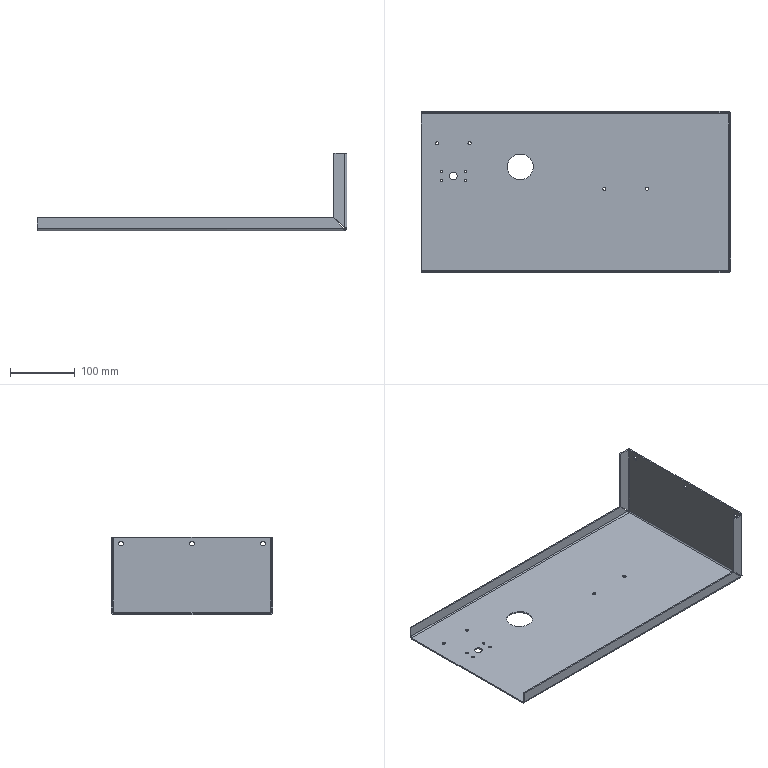Part | NX | features BREP 1 | 1 solid | 72 faces | box 480 x 250 x 120 mm | volume 333506 mm3 | cylinder 36 | plane 32 | spline 4 | commonest cylinder face diameters 4 x13 7 x6 8 x5 4.8 x4 5 x4 12 x2